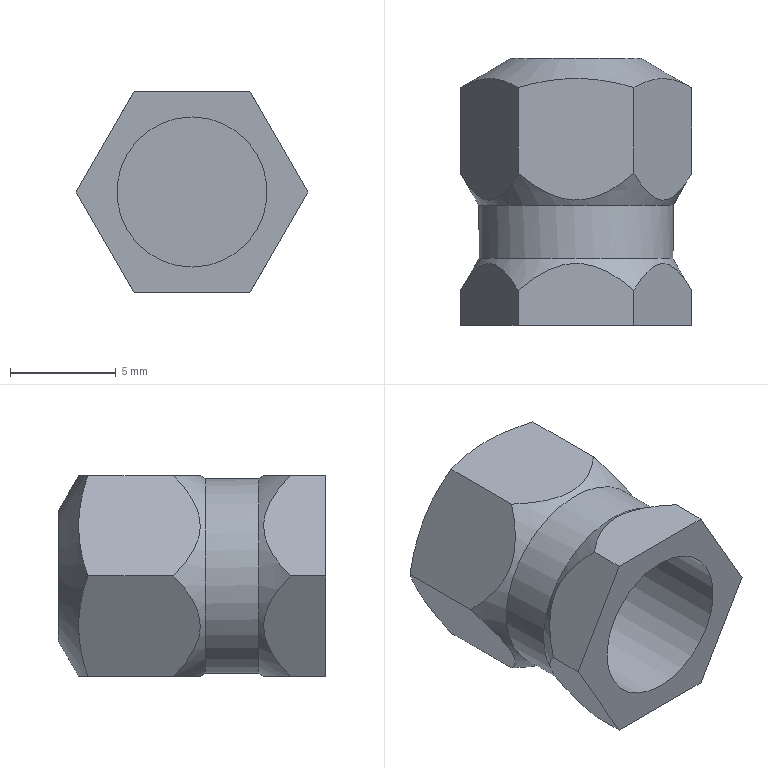Part | NX | features shrader MS20813-1 2 | 1 solid | 20 faces | box 10.969 x 12.649 x 9.5 mm | volume 618.121 mm3 | plane 15 | cone 3 | cylinder 2 | commonest cylinder face diameters 7.112 x1 9.22 x1
STEP:
#1=CARTESIAN_POINT('',(2.742,1.66,-4.75));
#2=VERTEX_POINT('',#1);
#3=CARTESIAN_POINT('',(2.742,0.,-4.75));
#4=VERTEX_POINT('',#3);
#5=CARTESIAN_POINT('',(2.742,12.649,-4.75));
#6=DIRECTION('',(0.,-1.,0.));
#7=VECTOR('',#6,1000.);
#8=LINE('',#5,#7);
#9=EDGE_CURVE('',#2,#4,#8,.T.);
#10=ORIENTED_EDGE('',*,*,#9,.F.);
#11=CARTESIAN_POINT('',(5.485,1.66,0.));
#12=VERTEX_POINT('',#11);
#13=CARTESIAN_POINT('',(2.742,1.66,-4.75));
#14=CARTESIAN_POINT('',(2.937,1.998,-4.412));
#15=CARTESIAN_POINT('',(3.344,2.615,-3.707));
#16=CARTESIAN_POINT('',(4.113,3.09,-2.375));
#17=CARTESIAN_POINT('',(4.875,2.623,-1.056));
#18=CARTESIAN_POINT('',(5.289,1.999,-0.3387));
#19=CARTESIAN_POINT('',(5.485,1.66,0.));
#20=B_SPLINE_CURVE_WITH_KNOTS('',3,(#13,#14,#15,#16,#17,#18,#19),.UNSPECIFIED.,.F.,.F.,(4,1,1,1,4),(0.000000303,0.001534,0.003068,0.004601,0.006135),.UNSPECIFIED.);
#21=EDGE_CURVE('',#2,#12,#20,.T.);
#22=ORIENTED_EDGE('',*,*,#21,.T.);
#23=CARTESIAN_POINT('',(5.485,0.,0.));
#24=VERTEX_POINT('',#23);
#25=CARTESIAN_POINT('',(5.485,12.649,0.));
#26=DIRECTION('',(0.,-1.,0.));
#27=VECTOR('',#26,1000.);
#28=LINE('',#25,#27);
#29=EDGE_CURVE('',#12,#24,#28,.T.);
#30=ORIENTED_EDGE('',*,*,#29,.T.);
#31=CARTESIAN_POINT('',(5.485,0.,0.));
#32=DIRECTION('',(-0.5,0.,-0.866));
#33=VECTOR('',#32,1000.);
#34=LINE('',#31,#33);
#35=EDGE_CURVE('',#24,#4,#34,.T.);
#36=ORIENTED_EDGE('',*,*,#35,.T.);
#37=EDGE_LOOP('',(#10,#22,#30,#36));
#38=FACE_BOUND('',#37,.T.);
#39=CARTESIAN_POINT('',(5.485,12.649,0.));
#40=DIRECTION('',(-0.866,0.,0.5));
#41=DIRECTION('',(0.5,0.,0.866));
#42=AXIS2_PLACEMENT_3D('',#39,#40,#41);
#43=PLANE('',#42);
#44=ADVANCED_FACE('',(#38),#43,.F.);
#45=CARTESIAN_POINT('',(-2.742,1.66,-4.75));
#46=VERTEX_POINT('',#45);
#47=CARTESIAN_POINT('',(-2.742,0.,-4.75));
#48=VERTEX_POINT('',#47);
#49=CARTESIAN_POINT('',(-2.742,12.649,-4.75));
#50=DIRECTION('',(0.,-1.,0.));
#51=VECTOR('',#50,1000.);
#52=LINE('',#49,#51);
#53=EDGE_CURVE('',#46,#48,#52,.T.);
#54=ORIENTED_EDGE('',*,*,#53,.F.);
#55=CARTESIAN_POINT('',(-2.742,1.66,-4.75));
#56=CARTESIAN_POINT('',(-2.357,1.994,-4.75));
#57=CARTESIAN_POINT('',(-1.53,2.62,-4.75));
#58=CARTESIAN_POINT('',(-0.00443,3.09,-4.75));
#59=CARTESIAN_POINT('',(1.532,2.62,-4.75));
#60=CARTESIAN_POINT('',(2.355,1.996,-4.75));
#61=CARTESIAN_POINT('',(2.742,1.66,-4.75));
#62=B_SPLINE_CURVE_WITH_KNOTS('',3,(#55,#56,#57,#58,#59,#60,#61),.UNSPECIFIED.,.F.,.F.,(4,1,1,1,4),(0.002746,0.004273,0.005799,0.007326,0.008853),.UNSPECIFIED.);
#63=EDGE_CURVE('',#46,#2,#62,.T.);
#64=ORIENTED_EDGE('',*,*,#63,.T.);
#65=ORIENTED_EDGE('',*,*,#9,.T.);
#66=CARTESIAN_POINT('',(2.742,0.,-4.75));
#67=DIRECTION('',(-1.,0.,0.));
#68=VECTOR('',#67,1000.);
#69=LINE('',#66,#68);
#70=EDGE_CURVE('',#4,#48,#69,.T.);
#71=ORIENTED_EDGE('',*,*,#70,.T.);
#72=EDGE_LOOP('',(#54,#64,#65,#71));
#73=FACE_BOUND('',#72,.T.);
#74=CARTESIAN_POINT('',(2.742,12.649,-4.75));
#75=DIRECTION('',(0.,0.,1.));
#76=DIRECTION('',(1.,0.,0.));
#77=AXIS2_PLACEMENT_3D('',#74,#75,#76);
#78=PLANE('',#77);
#79=ADVANCED_FACE('',(#73),#78,.F.);
#80=CARTESIAN_POINT('',(-5.485,1.66,0.));
#81=VERTEX_POINT('',#80);
#82=CARTESIAN_POINT('',(-5.485,0.,0.));
#83=VERTEX_POINT('',#82);
#84=CARTESIAN_POINT('',(-5.485,12.649,0.));
#85=DIRECTION('',(0.,-1.,0.));
#86=VECTOR('',#85,1000.);
#87=LINE('',#84,#86);
#88=EDGE_CURVE('',#81,#83,#87,.T.);
#89=ORIENTED_EDGE('',*,*,#88,.F.);
#90=CARTESIAN_POINT('',(-5.485,1.66,0.));
#91=CARTESIAN_POINT('',(-5.29,1.998,-0.3376));
#92=CARTESIAN_POINT('',(-4.882,2.615,-1.043));
#93=CARTESIAN_POINT('',(-4.113,3.09,-2.375));
#94=CARTESIAN_POINT('',(-3.352,2.623,-3.694));
#95=CARTESIAN_POINT('',(-2.938,1.999,-4.411));
#96=CARTESIAN_POINT('',(-2.742,1.66,-4.75));
#97=B_SPLINE_CURVE_WITH_KNOTS('',3,(#90,#91,#92,#93,#94,#95,#96),.UNSPECIFIED.,.F.,.F.,(4,1,1,1,4),(0.000000303,0.001534,0.003068,0.004601,0.006135),.UNSPECIFIED.);
#98=EDGE_CURVE('',#81,#46,#97,.T.);
#99=ORIENTED_EDGE('',*,*,#98,.T.);
#100=ORIENTED_EDGE('',*,*,#53,.T.);
#101=CARTESIAN_POINT('',(-2.742,0.,-4.75));
#102=DIRECTION('',(-0.5,0.,0.866));
#103=VECTOR('',#102,1000.);
#104=LINE('',#101,#103);
#105=EDGE_CURVE('',#48,#83,#104,.T.);
#106=ORIENTED_EDGE('',*,*,#105,.T.);
#107=EDGE_LOOP('',(#89,#99,#100,#106));
#108=FACE_BOUND('',#107,.T.);
#109=CARTESIAN_POINT('',(-2.742,12.649,-4.75));
#110=DIRECTION('',(0.866,0.,0.5));
#111=DIRECTION('',(0.5,0.,-0.866));
#112=AXIS2_PLACEMENT_3D('',#109,#110,#111);
#113=PLANE('',#112);
#114=ADVANCED_FACE('',(#108),#113,.F.);
#115=CARTESIAN_POINT('',(-2.742,1.66,4.75));
#116=VERTEX_POINT('',#115);
#117=CARTESIAN_POINT('',(-2.742,0.,4.75));
#118=VERTEX_POINT('',#117);
#119=CARTESIAN_POINT('',(-2.742,12.649,4.75));
#120=DIRECTION('',(0.,-1.,0.));
#121=VECTOR('',#120,1000.);
#122=LINE('',#119,#121);
#123=EDGE_CURVE('',#116,#118,#122,.T.);
#124=ORIENTED_EDGE('',*,*,#123,.F.);
#125=CARTESIAN_POINT('',(-2.742,1.66,4.75));
#126=CARTESIAN_POINT('',(-2.937,1.998,4.412));
#127=CARTESIAN_POINT('',(-3.344,2.615,3.707));
#128=CARTESIAN_POINT('',(-4.113,3.09,2.375));
#129=CARTESIAN_POINT('',(-4.875,2.623,1.056));
#130=CARTESIAN_POINT('',(-5.289,1.999,0.3387));
#131=CARTESIAN_POINT('',(-5.485,1.66,0.));
#132=B_SPLINE_CURVE_WITH_KNOTS('',3,(#125,#126,#127,#128,#129,#130,#131),.UNSPECIFIED.,.F.,.F.,(4,1,1,1,4),(0.000000303,0.001534,0.003068,0.004601,0.006135),.UNSPECIFIED.);
#133=EDGE_CURVE('',#116,#81,#132,.T.);
#134=ORIENTED_EDGE('',*,*,#133,.T.);
#135=ORIENTED_EDGE('',*,*,#88,.T.);
#136=CARTESIAN_POINT('',(-5.485,0.,0.));
#137=DIRECTION('',(0.5,0.,0.866));
#138=VECTOR('',#137,1000.);
#139=LINE('',#136,#138);
#140=EDGE_CURVE('',#83,#118,#139,.T.);
#141=ORIENTED_EDGE('',*,*,#140,.T.);
#142=EDGE_LOOP('',(#124,#134,#135,#141));
#143=FACE_BOUND('',#142,.T.);
#144=CARTESIAN_POINT('',(-5.485,12.649,0.));
#145=DIRECTION('',(0.866,0.,-0.5));
#146=DIRECTION('',(-0.5,0.,-0.866));
#147=AXIS2_PLACEMENT_3D('',#144,#145,#146);
#148=PLANE('',#147);
#149=ADVANCED_FACE('',(#143),#148,.F.);
#150=CARTESIAN_POINT('',(2.742,1.66,4.75));
#151=VERTEX_POINT('',#150);
#152=CARTESIAN_POINT('',(2.742,0.,4.75));
#153=VERTEX_POINT('',#152);
#154=CARTESIAN_POINT('',(2.742,12.649,4.75));
#155=DIRECTION('',(0.,-1.,0.));
#156=VECTOR('',#155,1000.);
#157=LINE('',#154,#156);
#158=EDGE_CURVE('',#151,#153,#157,.T.);
#159=ORIENTED_EDGE('',*,*,#158,.F.);
#160=CARTESIAN_POINT('',(-2.742,1.66,4.75));
#161=CARTESIAN_POINT('',(-2.357,1.994,4.75));
#162=CARTESIAN_POINT('',(-1.53,2.62,4.75));
#163=CARTESIAN_POINT('',(-0.00443,3.09,4.75));
#164=CARTESIAN_POINT('',(1.532,2.62,4.75));
#165=CARTESIAN_POINT('',(2.355,1.996,4.75));
#166=CARTESIAN_POINT('',(2.742,1.66,4.75));
#167=B_SPLINE_CURVE_WITH_KNOTS('',3,(#160,#161,#162,#163,#164,#165,#166),.UNSPECIFIED.,.F.,.F.,(4,1,1,1,4),(0.002746,0.004273,0.005799,0.007326,0.008853),.UNSPECIFIED.);
#168=EDGE_CURVE('',#151,#116,#167,.F.);
#169=ORIENTED_EDGE('',*,*,#168,.T.);
#170=ORIENTED_EDGE('',*,*,#123,.T.);
#171=CARTESIAN_POINT('',(-2.742,0.,4.75));
#172=DIRECTION('',(1.,0.,0.));
#173=VECTOR('',#172,1000.);
#174=LINE('',#171,#173);
#175=EDGE_CURVE('',#118,#153,#174,.T.);
#176=ORIENTED_EDGE('',*,*,#175,.T.);
#177=EDGE_LOOP('',(#159,#169,#170,#176));
#178=FACE_BOUND('',#177,.T.);
#179=CARTESIAN_POINT('',(-2.742,12.649,4.75));
#180=DIRECTION('',(0.,0.,-1.));
#181=DIRECTION('',(-1.,0.,0.));
#182=AXIS2_PLACEMENT_3D('',#179,#180,#181);
#183=PLANE('',#182);
#184=ADVANCED_FACE('',(#178),#183,.F.);
#185=ORIENTED_EDGE('',*,*,#29,.F.);
#186=CARTESIAN_POINT('',(5.485,1.66,0.));
#187=CARTESIAN_POINT('',(5.29,1.998,0.3376));
#188=CARTESIAN_POINT('',(4.882,2.615,1.043));
#189=CARTESIAN_POINT('',(4.113,3.09,2.375));
#190=CARTESIAN_POINT('',(3.352,2.623,3.694));
#191=CARTESIAN_POINT('',(2.938,1.999,4.411));
#192=CARTESIAN_POINT('',(2.742,1.66,4.75));
#193=B_SPLINE_CURVE_WITH_KNOTS('',3,(#186,#187,#188,#189,#190,#191,#192),.UNSPECIFIED.,.F.,.F.,(4,1,1,1,4),(0.000000303,0.001534,0.003068,0.004601,0.006135),.UNSPECIFIED.);
#194=EDGE_CURVE('',#12,#151,#193,.T.);
#195=ORIENTED_EDGE('',*,*,#194,.T.);
#196=ORIENTED_EDGE('',*,*,#158,.T.);
#197=CARTESIAN_POINT('',(2.742,0.,4.75));
#198=DIRECTION('',(0.5,0.,-0.866));
#199=VECTOR('',#198,1000.);
#200=LINE('',#197,#199);
#201=EDGE_CURVE('',#153,#24,#200,.T.);
#202=ORIENTED_EDGE('',*,*,#201,.T.);
#203=EDGE_LOOP('',(#185,#195,#196,#202));
#204=FACE_BOUND('',#203,.T.);
#205=CARTESIAN_POINT('',(2.742,12.649,4.75));
#206=DIRECTION('',(-0.866,0.,-0.5));
#207=DIRECTION('',(-0.5,0.,0.866));
#208=AXIS2_PLACEMENT_3D('',#205,#206,#207);
#209=PLANE('',#208);
#210=ADVANCED_FACE('',(#204),#209,.F.);
#211=CARTESIAN_POINT('',(0.,0.,-3.556));
#212=VERTEX_POINT('',#211);
#213=CARTESIAN_POINT('',(0.,0.,0.));
#214=DIRECTION('',(0.,-1.,0.));
#215=DIRECTION('',(0.,0.,-1.));
#216=AXIS2_PLACEMENT_3D('',#213,#214,#215);
#217=CIRCLE('',#216,3.556);
#218=EDGE_CURVE('',#212,#212,#217,.T.);
#219=ORIENTED_EDGE('',*,*,#218,.F.);
#220=EDGE_LOOP('',(#219));
#221=FACE_BOUND('',#220,.T.);
#222=ORIENTED_EDGE('',*,*,#35,.F.);
#223=ORIENTED_EDGE('',*,*,#201,.F.);
#224=ORIENTED_EDGE('',*,*,#175,.F.);
#225=ORIENTED_EDGE('',*,*,#140,.F.);
#226=ORIENTED_EDGE('',*,*,#105,.F.);
#227=ORIENTED_EDGE('',*,*,#70,.F.);
#228=EDGE_LOOP('',(#222,#223,#224,#225,#226,#227));
#229=FACE_BOUND('',#228,.T.);
#230=CARTESIAN_POINT('',(2.742,0.,-4.75));
#231=DIRECTION('',(0.,1.,0.));
#232=DIRECTION('',(0.,0.,1.));
#233=AXIS2_PLACEMENT_3D('',#230,#231,#232);
#234=PLANE('',#233);
#235=ADVANCED_FACE('',(#221,#229),#234,.F.);
#236=CARTESIAN_POINT('',(0.,5.69,-4.61));
#237=VERTEX_POINT('',#236);
#238=CARTESIAN_POINT('',(0.,5.69,0.));
#239=DIRECTION('',(0.,-1.,0.));
#240=DIRECTION('',(0.,0.,-1.));
#241=AXIS2_PLACEMENT_3D('',#238,#239,#240);
#242=CIRCLE('',#241,4.61);
#243=EDGE_CURVE('',#237,#237,#242,.T.);
#244=ORIENTED_EDGE('',*,*,#243,.F.);
#245=EDGE_LOOP('',(#244));
#246=FACE_BOUND('',#245,.T.);
#247=CARTESIAN_POINT('',(2.742,7.204,4.75));
#248=VERTEX_POINT('',#247);
#249=CARTESIAN_POINT('',(5.485,7.204,0.));
#250=VERTEX_POINT('',#249);
#251=CARTESIAN_POINT('',(2.742,7.204,4.75));
#252=CARTESIAN_POINT('',(2.937,6.867,4.412));
#253=CARTESIAN_POINT('',(3.344,6.249,3.707));
#254=CARTESIAN_POINT('',(4.113,5.775,2.375));
#255=CARTESIAN_POINT('',(4.875,6.242,1.056));
#256=CARTESIAN_POINT('',(5.289,6.866,0.3387));
#257=CARTESIAN_POINT('',(5.485,7.204,0.));
#258=B_SPLINE_CURVE_WITH_KNOTS('',3,(#251,#252,#253,#254,#255,#256,#257),.UNSPECIFIED.,.F.,.F.,(4,1,1,1,4),(0.000000303,0.001534,0.003068,0.004601,0.006135),.UNSPECIFIED.);
#259=EDGE_CURVE('',#248,#250,#258,.T.);
#260=ORIENTED_EDGE('',*,*,#259,.F.);
#261=CARTESIAN_POINT('',(-2.742,7.204,4.75));
#262=VERTEX_POINT('',#261);
#263=CARTESIAN_POINT('',(-2.742,7.204,4.75));
#264=CARTESIAN_POINT('',(-2.357,6.871,4.75));
#265=CARTESIAN_POINT('',(-1.53,6.245,4.75));
#266=CARTESIAN_POINT('',(-0.00443,5.775,4.75));
#267=CARTESIAN_POINT('',(1.532,6.245,4.75));
#268=CARTESIAN_POINT('',(2.355,6.869,4.75));
#269=CARTESIAN_POINT('',(2.742,7.204,4.75));
#270=B_SPLINE_CURVE_WITH_KNOTS('',3,(#263,#264,#265,#266,#267,#268,#269),.UNSPECIFIED.,.F.,.F.,(4,1,1,1,4),(0.002746,0.004273,0.005799,0.007326,0.008853),.UNSPECIFIED.);
#271=EDGE_CURVE('',#262,#248,#270,.T.);
#272=ORIENTED_EDGE('',*,*,#271,.F.);
#273=CARTESIAN_POINT('',(-5.485,7.204,0.));
#274=VERTEX_POINT('',#273);
#275=CARTESIAN_POINT('',(-5.485,7.204,0.));
#276=CARTESIAN_POINT('',(-5.29,6.867,0.3376));
#277=CARTESIAN_POINT('',(-4.882,6.249,1.043));
#278=CARTESIAN_POINT('',(-4.113,5.775,2.375));
#279=CARTESIAN_POINT('',(-3.352,6.242,3.694));
#280=CARTESIAN_POINT('',(-2.938,6.866,4.411));
#281=CARTESIAN_POINT('',(-2.742,7.204,4.75));
#282=B_SPLINE_CURVE_WITH_KNOTS('',3,(#275,#276,#277,#278,#279,#280,#281),.UNSPECIFIED.,.F.,.F.,(4,1,1,1,4),(0.000000303,0.001534,0.003068,0.004601,0.006135),.UNSPECIFIED.);
#283=EDGE_CURVE('',#274,#262,#282,.T.);
#284=ORIENTED_EDGE('',*,*,#283,.F.);
#285=CARTESIAN_POINT('',(-2.742,7.204,-4.75));
#286=VERTEX_POINT('',#285);
#287=CARTESIAN_POINT('',(-2.742,7.204,-4.75));
#288=CARTESIAN_POINT('',(-2.937,6.867,-4.412));
#289=CARTESIAN_POINT('',(-3.344,6.249,-3.707));
#290=CARTESIAN_POINT('',(-4.113,5.775,-2.375));
#291=CARTESIAN_POINT('',(-4.875,6.242,-1.056));
#292=CARTESIAN_POINT('',(-5.289,6.866,-0.3387));
#293=CARTESIAN_POINT('',(-5.485,7.204,0.));
#294=B_SPLINE_CURVE_WITH_KNOTS('',3,(#287,#288,#289,#290,#291,#292,#293),.UNSPECIFIED.,.F.,.F.,(4,1,1,1,4),(0.000000303,0.001534,0.003068,0.004601,0.006135),.UNSPECIFIED.);
#295=EDGE_CURVE('',#286,#274,#294,.T.);
#296=ORIENTED_EDGE('',*,*,#295,.F.);
#297=CARTESIAN_POINT('',(2.742,7.204,-4.75));
#298=VERTEX_POINT('',#297);
#299=CARTESIAN_POINT('',(-2.742,7.204,-4.75));
#300=CARTESIAN_POINT('',(-2.357,6.871,-4.75));
#301=CARTESIAN_POINT('',(-1.53,6.245,-4.75));
#302=CARTESIAN_POINT('',(-0.00443,5.775,-4.75));
#303=CARTESIAN_POINT('',(1.532,6.245,-4.75));
#304=CARTESIAN_POINT('',(2.355,6.869,-4.75));
#305=CARTESIAN_POINT('',(2.742,7.204,-4.75));
#306=B_SPLINE_CURVE_WITH_KNOTS('',3,(#299,#300,#301,#302,#303,#304,#305),.UNSPECIFIED.,.F.,.F.,(4,1,1,1,4),(0.002746,0.004273,0.005799,0.007326,0.008853),.UNSPECIFIED.);
#307=EDGE_CURVE('',#298,#286,#306,.F.);
#308=ORIENTED_EDGE('',*,*,#307,.F.);
#309=CARTESIAN_POINT('',(5.485,7.204,0.));
#310=CARTESIAN_POINT('',(5.29,6.867,-0.3376));
#311=CARTESIAN_POINT('',(4.882,6.249,-1.043));
#312=CARTESIAN_POINT('',(4.113,5.775,-2.375));
#313=CARTESIAN_POINT('',(3.352,6.242,-3.694));
#314=CARTESIAN_POINT('',(2.938,6.866,-4.411));
#315=CARTESIAN_POINT('',(2.742,7.204,-4.75));
#316=B_SPLINE_CURVE_WITH_KNOTS('',3,(#309,#310,#311,#312,#313,#314,#315),.UNSPECIFIED.,.F.,.F.,(4,1,1,1,4),(0.000000303,0.001534,0.003068,0.004601,0.006135),.UNSPECIFIED.);
#317=EDGE_CURVE('',#250,#298,#316,.T.);
#318=ORIENTED_EDGE('',*,*,#317,.F.);
#319=EDGE_LOOP('',(#260,#272,#284,#296,#308,#318));
#320=FACE_BOUND('',#319,.T.);
#321=CARTESIAN_POINT('',(0.,7.204,0.));
#322=DIRECTION('',(0.,1.,0.));
#323=DIRECTION('',(0.,0.,1.));
#324=AXIS2_PLACEMENT_3D('',#321,#322,#323);
#325=CONICAL_SURFACE('',#324,5.485,0.5236);
#326=ADVANCED_FACE('',(#246,#320),#325,.T.);
#327=CARTESIAN_POINT('',(0.,3.175,-4.61));
#328=VERTEX_POINT('',#327);
#329=CARTESIAN_POINT('',(0.,3.175,0.));
#330=DIRECTION('',(0.,-1.,0.));
#331=DIRECTION('',(0.,0.,-1.));
#332=AXIS2_PLACEMENT_3D('',#329,#330,#331);
#333=CIRCLE('',#332,4.61);
#334=EDGE_CURVE('',#328,#328,#333,.T.);
#335=ORIENTED_EDGE('',*,*,#334,.T.);
#336=EDGE_LOOP('',(#335));
#337=FACE_BOUND('',#336,.T.);
#338=ORIENTED_EDGE('',*,*,#63,.F.);
#339=ORIENTED_EDGE('',*,*,#98,.F.);
#340=ORIENTED_EDGE('',*,*,#133,.F.);
#341=ORIENTED_EDGE('',*,*,#168,.F.);
#342=ORIENTED_EDGE('',*,*,#194,.F.);
#343=ORIENTED_EDGE('',*,*,#21,.F.);
#344=EDGE_LOOP('',(#338,#339,#340,#341,#342,#343));
#345=FACE_BOUND('',#344,.T.);
#346=CARTESIAN_POINT('',(0.,3.175,0.));
#347=DIRECTION('',(0.,-1.,0.));
#348=DIRECTION('',(0.,0.,-1.));
#349=AXIS2_PLACEMENT_3D('',#346,#347,#348);
#350=CONICAL_SURFACE('',#349,4.61,0.5236);
#351=ADVANCED_FACE('',(#337,#345),#350,.T.);
#352=ORIENTED_EDGE('',*,*,#334,.F.);
#353=EDGE_LOOP('',(#352));
#354=FACE_BOUND('',#353,.T.);
#355=ORIENTED_EDGE('',*,*,#243,.T.);
#356=EDGE_LOOP('',(#355));
#357=FACE_BOUND('',#356,.T.);
#358=CARTESIAN_POINT('',(0.,7.62,0.));
#359=DIRECTION('',(0.,-1.,0.));
#360=DIRECTION('',(0.,0.,-1.));
#361=AXIS2_PLACEMENT_3D('',#358,#359,#360);
#362=CYLINDRICAL_SURFACE('',#361,4.61);
#363=ADVANCED_FACE('',(#354,#357),#362,.T.);
#364=CARTESIAN_POINT('',(5.485,11.264,0.));
#365=VERTEX_POINT('',#364);
#366=CARTESIAN_POINT('',(5.485,12.649,0.));
#367=DIRECTION('',(0.,-1.,0.));
#368=VECTOR('',#367,1000.);
#369=LINE('',#366,#368);
#370=EDGE_CURVE('',#365,#250,#369,.T.);
#371=ORIENTED_EDGE('',*,*,#370,.F.);
#372=CARTESIAN_POINT('',(2.742,11.264,4.75));
#373=VERTEX_POINT('',#372);
#374=CARTESIAN_POINT('',(5.485,11.264,0.));
#375=CARTESIAN_POINT('',(5.037,11.523,0.7756));
#376=CARTESIAN_POINT('',(4.118,11.854,2.366));
#377=CARTESIAN_POINT('',(3.191,11.523,3.973));
#378=CARTESIAN_POINT('',(2.742,11.264,4.75));
#379=B_SPLINE_CURVE_WITH_KNOTS('',3,(#374,#375,#376,#377,#378),.UNSPECIFIED.,.F.,.F.,(4,1,4),(0.000000238,0.00277,0.005539),.UNSPECIFIED.);
#380=EDGE_CURVE('',#365,#373,#379,.T.);
#381=ORIENTED_EDGE('',*,*,#380,.T.);
#382=CARTESIAN_POINT('',(2.742,12.649,4.75));
#383=DIRECTION('',(0.,-1.,0.));
#384=VECTOR('',#383,1000.);
#385=LINE('',#382,#384);
#386=EDGE_CURVE('',#373,#248,#385,.T.);
#387=ORIENTED_EDGE('',*,*,#386,.T.);
#388=ORIENTED_EDGE('',*,*,#259,.T.);
#389=EDGE_LOOP('',(#371,#381,#387,#388));
#390=FACE_BOUND('',#389,.T.);
#391=CARTESIAN_POINT('',(2.742,12.649,4.75));
#392=DIRECTION('',(-0.866,0.,-0.5));
#393=DIRECTION('',(-0.5,0.,0.866));
#394=AXIS2_PLACEMENT_3D('',#391,#392,#393);
#395=PLANE('',#394);
#396=ADVANCED_FACE('',(#390),#395,.F.);
#397=ORIENTED_EDGE('',*,*,#386,.F.);
#398=CARTESIAN_POINT('',(-2.742,11.264,4.75));
#399=VERTEX_POINT('',#398);
#400=CARTESIAN_POINT('',(-2.742,11.264,4.75));
#401=CARTESIAN_POINT('',(-1.851,11.522,4.75));
#402=CARTESIAN_POINT('',(-0.001093,11.856,4.75));
#403=CARTESIAN_POINT('',(1.856,11.52,4.75));
#404=CARTESIAN_POINT('',(2.742,11.264,4.75));
#405=B_SPLINE_CURVE_WITH_KNOTS('',3,(#400,#401,#402,#403,#404),.UNSPECIFIED.,.F.,.F.,(4,1,4),(0.004746,0.007519,0.01029),.UNSPECIFIED.);
#406=EDGE_CURVE('',#373,#399,#405,.F.);
#407=ORIENTED_EDGE('',*,*,#406,.T.);
#408=CARTESIAN_POINT('',(-2.742,12.649,4.75));
#409=DIRECTION('',(0.,-1.,0.));
#410=VECTOR('',#409,1000.);
#411=LINE('',#408,#410);
#412=EDGE_CURVE('',#399,#262,#411,.T.);
#413=ORIENTED_EDGE('',*,*,#412,.T.);
#414=ORIENTED_EDGE('',*,*,#271,.T.);
#415=EDGE_LOOP('',(#397,#407,#413,#414));
#416=FACE_BOUND('',#415,.T.);
#417=CARTESIAN_POINT('',(-2.742,12.649,4.75));
#418=DIRECTION('',(0.,0.,-1.));
#419=DIRECTION('',(-1.,0.,0.));
#420=AXIS2_PLACEMENT_3D('',#417,#418,#419);
#421=PLANE('',#420);
#422=ADVANCED_FACE('',(#416),#421,.F.);
#423=ORIENTED_EDGE('',*,*,#412,.F.);
#424=CARTESIAN_POINT('',(-5.485,11.264,0.));
#425=VERTEX_POINT('',#424);
#426=CARTESIAN_POINT('',(-2.742,11.264,4.75));
#427=CARTESIAN_POINT('',(-3.19,11.523,3.974));
#428=CARTESIAN_POINT('',(-4.108,11.854,2.383));
#429=CARTESIAN_POINT('',(-5.036,11.523,0.7765));
#430=CARTESIAN_POINT('',(-5.485,11.264,0.));
#431=B_SPLINE_CURVE_WITH_KNOTS('',3,(#426,#427,#428,#429,#430),.UNSPECIFIED.,.F.,.F.,(4,1,4),(0.000000238,0.00277,0.005539),.UNSPECIFIED.);
#432=EDGE_CURVE('',#399,#425,#431,.T.);
#433=ORIENTED_EDGE('',*,*,#432,.T.);
#434=CARTESIAN_POINT('',(-5.485,12.649,0.));
#435=DIRECTION('',(0.,-1.,0.));
#436=VECTOR('',#435,1000.);
#437=LINE('',#434,#436);
#438=EDGE_CURVE('',#425,#274,#437,.T.);
#439=ORIENTED_EDGE('',*,*,#438,.T.);
#440=ORIENTED_EDGE('',*,*,#283,.T.);
#441=EDGE_LOOP('',(#423,#433,#439,#440));
#442=FACE_BOUND('',#441,.T.);
#443=CARTESIAN_POINT('',(-5.485,12.649,0.));
#444=DIRECTION('',(0.866,0.,-0.5));
#445=DIRECTION('',(-0.5,0.,-0.866));
#446=AXIS2_PLACEMENT_3D('',#443,#444,#445);
#447=PLANE('',#446);
#448=ADVANCED_FACE('',(#442),#447,.F.);
#449=ORIENTED_EDGE('',*,*,#438,.F.);
#450=CARTESIAN_POINT('',(-2.742,11.264,-4.75));
#451=VERTEX_POINT('',#450);
#452=CARTESIAN_POINT('',(-5.485,11.264,0.));
#453=CARTESIAN_POINT('',(-5.037,11.523,-0.7756));
#454=CARTESIAN_POINT('',(-4.118,11.854,-2.366));
#455=CARTESIAN_POINT('',(-3.191,11.523,-3.973));
#456=CARTESIAN_POINT('',(-2.742,11.264,-4.75));
#457=B_SPLINE_CURVE_WITH_KNOTS('',3,(#452,#453,#454,#455,#456),.UNSPECIFIED.,.F.,.F.,(4,1,4),(0.000000238,0.00277,0.005539),.UNSPECIFIED.);
#458=EDGE_CURVE('',#425,#451,#457,.T.);
#459=ORIENTED_EDGE('',*,*,#458,.T.);
#460=CARTESIAN_POINT('',(-2.742,12.649,-4.75));
#461=DIRECTION('',(0.,-1.,0.));
#462=VECTOR('',#461,1000.);
#463=LINE('',#460,#462);
#464=EDGE_CURVE('',#451,#286,#463,.T.);
#465=ORIENTED_EDGE('',*,*,#464,.T.);
#466=ORIENTED_EDGE('',*,*,#295,.T.);
#467=EDGE_LOOP('',(#449,#459,#465,#466));
#468=FACE_BOUND('',#467,.T.);
#469=CARTESIAN_POINT('',(-2.742,12.649,-4.75));
#470=DIRECTION('',(0.866,0.,0.5));
#471=DIRECTION('',(0.5,0.,-0.866));
#472=AXIS2_PLACEMENT_3D('',#469,#470,#471);
#473=PLANE('',#472);
#474=ADVANCED_FACE('',(#468),#473,.F.);
#475=ORIENTED_EDGE('',*,*,#464,.F.);
#476=CARTESIAN_POINT('',(2.742,11.264,-4.75));
#477=VERTEX_POINT('',#476);
#478=CARTESIAN_POINT('',(-2.742,11.264,-4.75));
#479=CARTESIAN_POINT('',(-1.851,11.522,-4.75));
#480=CARTESIAN_POINT('',(-0.001093,11.856,-4.75));
#481=CARTESIAN_POINT('',(1.856,11.52,-4.75));
#482=CARTESIAN_POINT('',(2.742,11.264,-4.75));
#483=B_SPLINE_CURVE_WITH_KNOTS('',3,(#478,#479,#480,#481,#482),.UNSPECIFIED.,.F.,.F.,(4,1,4),(0.004746,0.007519,0.01029),.UNSPECIFIED.);
#484=EDGE_CURVE('',#451,#477,#483,.T.);
#485=ORIENTED_EDGE('',*,*,#484,.T.);
#486=CARTESIAN_POINT('',(2.742,12.649,-4.75));
#487=DIRECTION('',(0.,-1.,0.));
#488=VECTOR('',#487,1000.);
#489=LINE('',#486,#488);
#490=EDGE_CURVE('',#477,#298,#489,.T.);
#491=ORIENTED_EDGE('',*,*,#490,.T.);
#492=ORIENTED_EDGE('',*,*,#307,.T.);
#493=EDGE_LOOP('',(#475,#485,#491,#492));
#494=FACE_BOUND('',#493,.T.);
#495=CARTESIAN_POINT('',(2.742,12.649,-4.75));
#496=DIRECTION('',(0.,0.,1.));
#497=DIRECTION('',(1.,0.,0.));
#498=AXIS2_PLACEMENT_3D('',#495,#496,#497);
#499=PLANE('',#498);
#500=ADVANCED_FACE('',(#494),#499,.F.);
#501=ORIENTED_EDGE('',*,*,#490,.F.);
#502=CARTESIAN_POINT('',(2.742,11.264,-4.75));
#503=CARTESIAN_POINT('',(3.19,11.523,-3.974));
#504=CARTESIAN_POINT('',(4.108,11.854,-2.383));
#505=CARTESIAN_POINT('',(5.036,11.523,-0.7765));
#506=CARTESIAN_POINT('',(5.485,11.264,0.));
#507=B_SPLINE_CURVE_WITH_KNOTS('',3,(#502,#503,#504,#505,#506),.UNSPECIFIED.,.F.,.F.,(4,1,4),(0.000000238,0.00277,0.005539),.UNSPECIFIED.);
#508=EDGE_CURVE('',#477,#365,#507,.T.);
#509=ORIENTED_EDGE('',*,*,#508,.T.);
#510=ORIENTED_EDGE('',*,*,#370,.T.);
#511=ORIENTED_EDGE('',*,*,#317,.T.);
#512=EDGE_LOOP('',(#501,#509,#510,#511));
#513=FACE_BOUND('',#512,.T.);
#514=CARTESIAN_POINT('',(5.485,12.649,0.));
#515=DIRECTION('',(-0.866,0.,0.5));
#516=DIRECTION('',(0.5,0.,0.866));
#517=AXIS2_PLACEMENT_3D('',#514,#515,#516);
#518=PLANE('',#517);
#519=ADVANCED_FACE('',(#513),#518,.F.);
#520=CARTESIAN_POINT('',(0.,12.649,-3.086));
#521=VERTEX_POINT('',#520);
#522=CARTESIAN_POINT('',(0.,12.649,0.));
#523=DIRECTION('',(0.,-1.,0.));
#524=DIRECTION('',(0.,0.,-1.));
#525=AXIS2_PLACEMENT_3D('',#522,#523,#524);
#526=CIRCLE('',#525,3.086);
#527=EDGE_CURVE('',#521,#521,#526,.T.);
#528=ORIENTED_EDGE('',*,*,#527,.T.);
#529=EDGE_LOOP('',(#528));
#530=FACE_BOUND('',#529,.T.);
#531=ORIENTED_EDGE('',*,*,#484,.F.);
#532=ORIENTED_EDGE('',*,*,#458,.F.);
#533=ORIENTED_EDGE('',*,*,#432,.F.);
#534=ORIENTED_EDGE('',*,*,#406,.F.);
#535=ORIENTED_EDGE('',*,*,#380,.F.);
#536=ORIENTED_EDGE('',*,*,#508,.F.);
#537=EDGE_LOOP('',(#531,#532,#533,#534,#535,#536));
#538=FACE_BOUND('',#537,.T.);
#539=CARTESIAN_POINT('',(0.,12.649,0.));
#540=DIRECTION('',(0.,-1.,0.));
#541=DIRECTION('',(0.,0.,-1.));
#542=AXIS2_PLACEMENT_3D('',#539,#540,#541);
#543=CONICAL_SURFACE('',#542,3.086,1.047);
#544=ADVANCED_FACE('',(#530,#538),#543,.T.);
#545=ORIENTED_EDGE('',*,*,#527,.F.);
#546=EDGE_LOOP('',(#545));
#547=FACE_BOUND('',#546,.T.);
#548=CARTESIAN_POINT('',(2.742,12.649,-4.75));
#549=DIRECTION('',(0.,1.,0.));
#550=DIRECTION('',(0.,0.,1.));
#551=AXIS2_PLACEMENT_3D('',#548,#549,#550);
#552=PLANE('',#551);
#553=ADVANCED_FACE('',(#547),#552,.T.);
#554=CARTESIAN_POINT('',(0.,7.62,-3.556));
#555=VERTEX_POINT('',#554);
#556=CARTESIAN_POINT('',(0.,7.62,0.));
#557=DIRECTION('',(0.,-1.,0.));
#558=DIRECTION('',(0.,0.,-1.));
#559=AXIS2_PLACEMENT_3D('',#556,#557,#558);
#560=CIRCLE('',#559,3.556);
#561=EDGE_CURVE('',#555,#555,#560,.T.);
#562=ORIENTED_EDGE('',*,*,#561,.F.);
#563=EDGE_LOOP('',(#562));
#564=FACE_BOUND('',#563,.T.);
#565=ORIENTED_EDGE('',*,*,#218,.T.);
#566=EDGE_LOOP('',(#565));
#567=FACE_BOUND('',#566,.T.);
#568=CARTESIAN_POINT('',(0.,7.62,0.));
#569=DIRECTION('',(0.,-1.,0.));
#570=DIRECTION('',(0.,0.,-1.));
#571=AXIS2_PLACEMENT_3D('',#568,#569,#570);
#572=CYLINDRICAL_SURFACE('',#571,3.556);
#573=ADVANCED_FACE('',(#564,#567),#572,.F.);
#574=ORIENTED_EDGE('',*,*,#561,.T.);
#575=EDGE_LOOP('',(#574));
#576=FACE_BOUND('',#575,.T.);
#577=CARTESIAN_POINT('',(3.556,7.62,0.));
#578=DIRECTION('',(0.,1.,0.));
#579=DIRECTION('',(0.,0.,1.));
#580=AXIS2_PLACEMENT_3D('',#577,#578,#579);
#581=PLANE('',#580);
#582=ADVANCED_FACE('',(#576),#581,.F.);
#583=CLOSED_SHELL('',(#44,#79,#114,#149,#184,#210,#235,#326,#351,#363,#396,#422,#448,#474,#500,#519,#544,#553,#573,#582));
#584=MANIFOLD_SOLID_BREP('',#583);
#585=(LENGTH_UNIT()NAMED_UNIT(*)SI_UNIT(.MILLI.,.METRE.));
#586=UNCERTAINTY_MEASURE_WITH_UNIT(LENGTH_MEASURE(0.0508),#585,'','');
#587=(NAMED_UNIT(*)PLANE_ANGLE_UNIT()SI_UNIT($,.RADIAN.));
#588=(NAMED_UNIT(*)SI_UNIT($,.STERADIAN.)SOLID_ANGLE_UNIT());
#589=(GEOMETRIC_REPRESENTATION_CONTEXT(3)GLOBAL_UNCERTAINTY_ASSIGNED_CONTEXT((#586))GLOBAL_UNIT_ASSIGNED_CONTEXT((#585,#587,#588))REPRESENTATION_CONTEXT('',''));
#590=ADVANCED_BREP_SHAPE_REPRESENTATION('',(#584),#589);